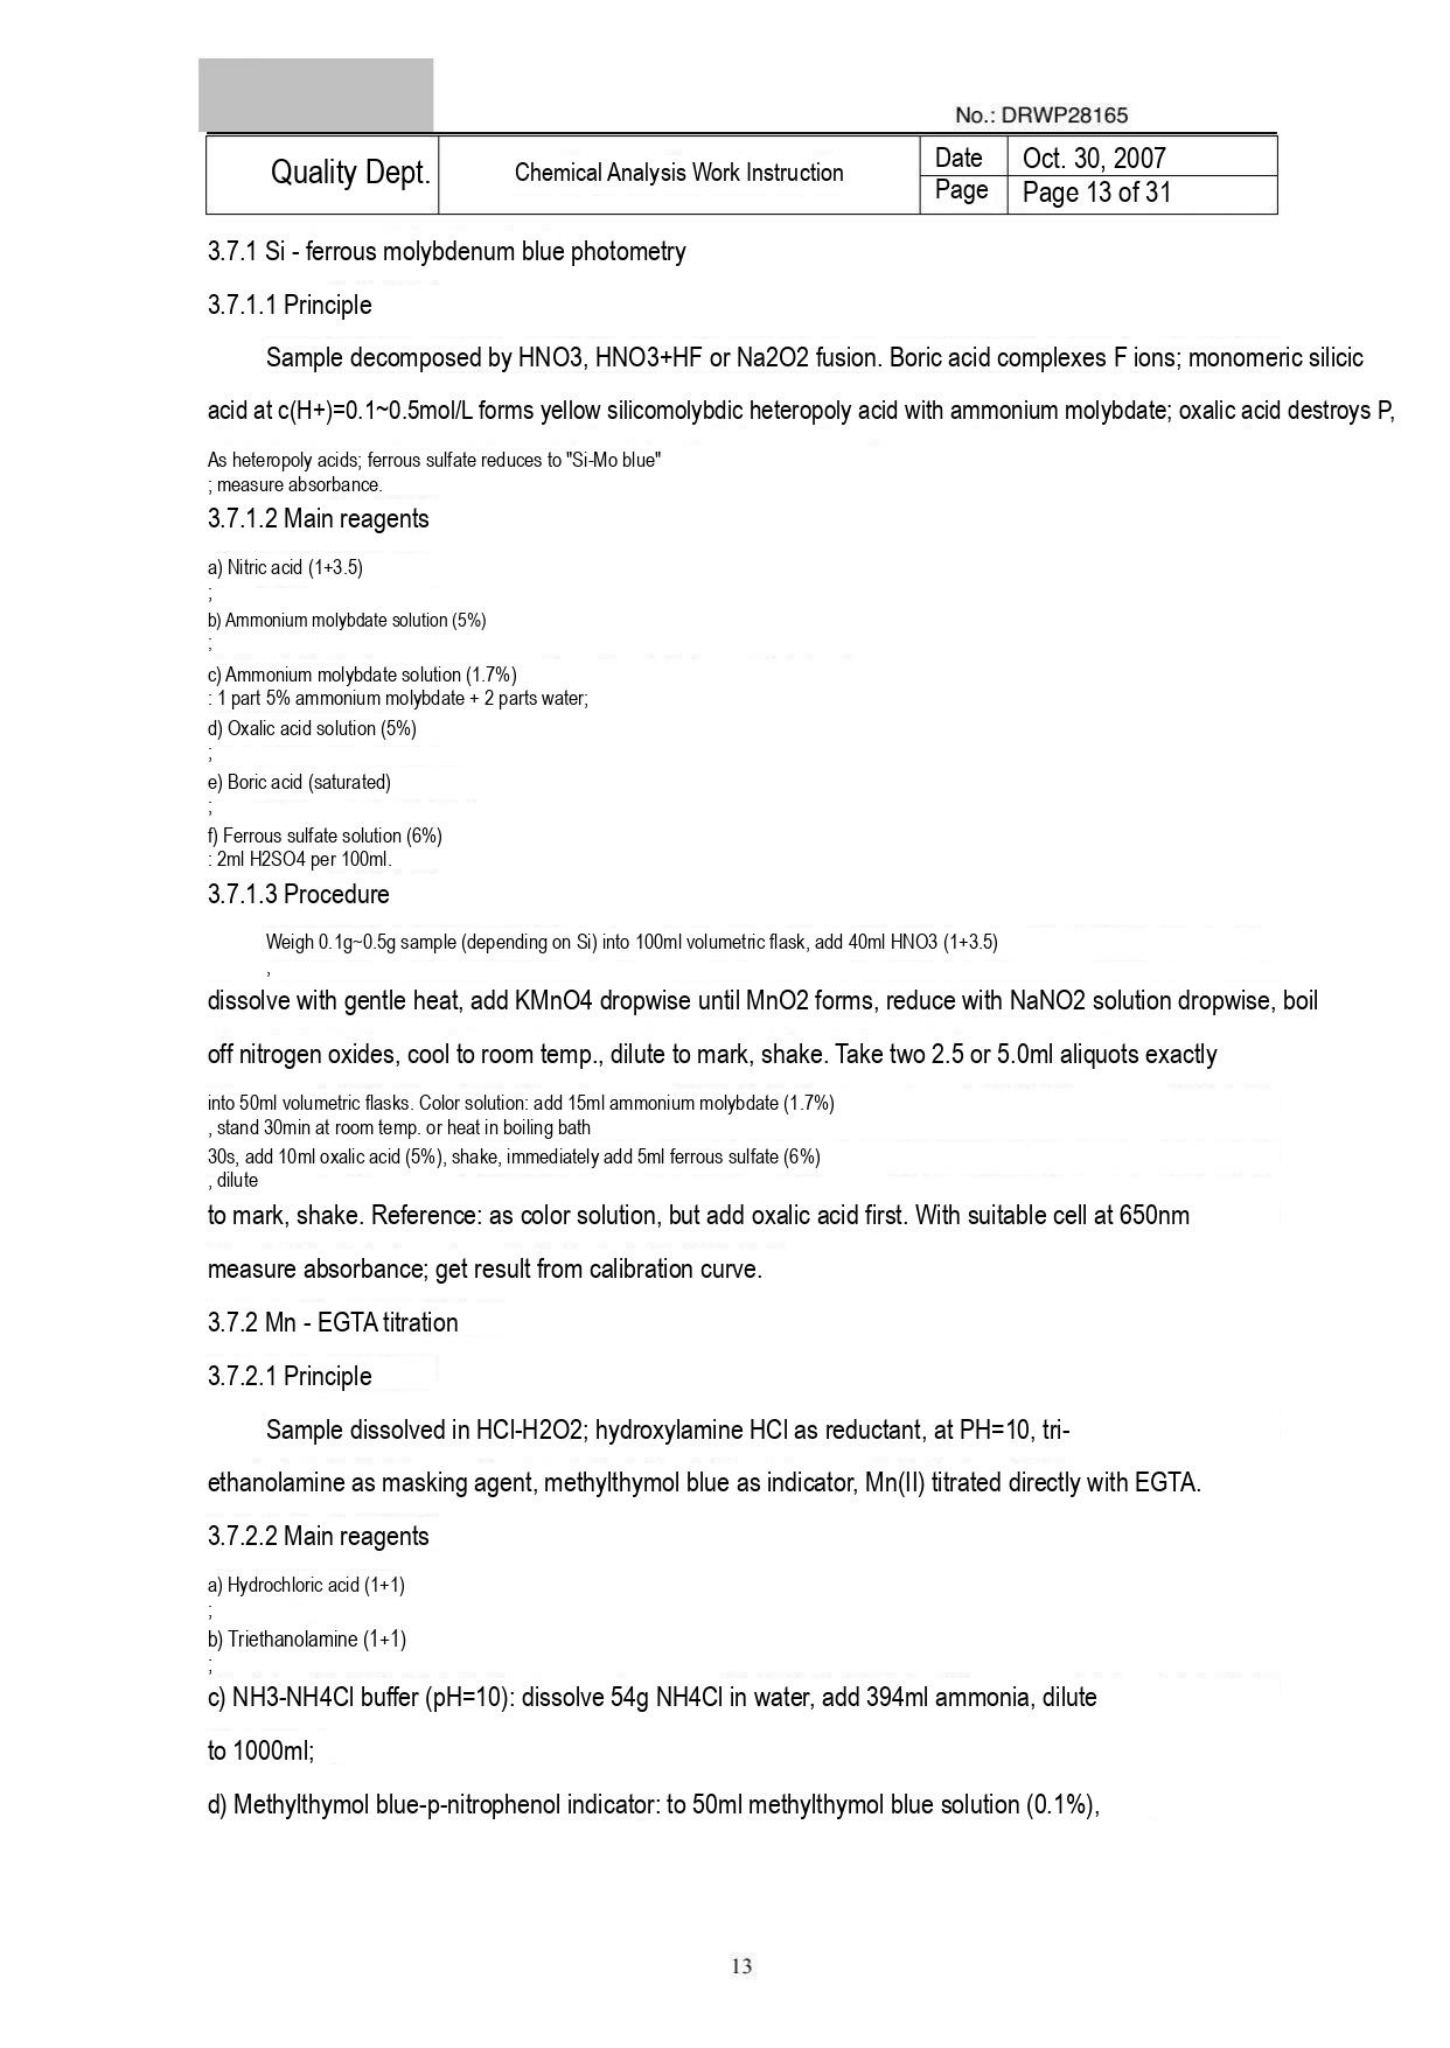No.: DRWP28165

| Quality Dept. | Chemical Analysis Work Instruction | Date | Oct. 30, 2007 |
|---|---|---|---|
| | | Page | Page 13 of 31 |

3.7.1 Si - ferrous molybdenum blue photometry

3.7.1.1 Principle

Sample decomposed by HNO3, HNO3+HF or Na2O2 fusion. Boric acid complexes F ions; monomeric silicic acid at c(H+)=0.1~0.5mol/L forms yellow silicomolybdic heteropoly acid with ammonium molybdate; oxalic acid destroys P, As heteropoly acids; ferrous sulfate reduces to "Si-Mo blue"
; measure absorbance.

3.7.1.2 Main reagents

a) Nitric acid (1+3.5)
;
b) Ammonium molybdate solution (5%)
;
c) Ammonium molybdate solution (1.7%)
: 1 part 5% ammonium molybdate + 2 parts water;
d) Oxalic acid solution (5%)
;
e) Boric acid (saturated)
;
f) Ferrous sulfate solution (6%)
: 2ml H2SO4 per 100ml.

3.7.1.3 Procedure

Weigh 0.1g~0.5g sample (depending on Si) into 100ml volumetric flask, add 40ml HNO3 (1+3.5)
,
dissolve with gentle heat, add KMnO4 dropwise until MnO2 forms, reduce with NaNO2 solution dropwise, boil off nitrogen oxides, cool to room temp., dilute to mark, shake. Take two 2.5 or 5.0ml aliquots exactly into 50ml volumetric flasks. Color solution: add 15ml ammonium molybdate (1.7%)
, stand 30min at room temp. or heat in boiling bath
30s, add 10ml oxalic acid (5%), shake, immediately add 5ml ferrous sulfate (6%)
, dilute
to mark, shake. Reference: as color solution, but add oxalic acid first. With suitable cell at 650nm measure absorbance; get result from calibration curve.

3.7.2 Mn - EGTA titration

3.7.2.1 Principle

Sample dissolved in HCl-H2O2; hydroxylamine HCl as reductant, at PH=10, tri-ethanolamine as masking agent, methylthymol blue as indicator, Mn(II) titrated directly with EGTA.

3.7.2.2 Main reagents

a) Hydrochloric acid (1+1)
;
b) Triethanolamine (1+1)
;
c) NH3-NH4Cl buffer (pH=10): dissolve 54g NH4Cl in water, add 394ml ammonia, dilute to 1000ml;

d) Methylthymol blue-p-nitrophenol indicator: to 50ml methylthymol blue solution (0.1%),

13
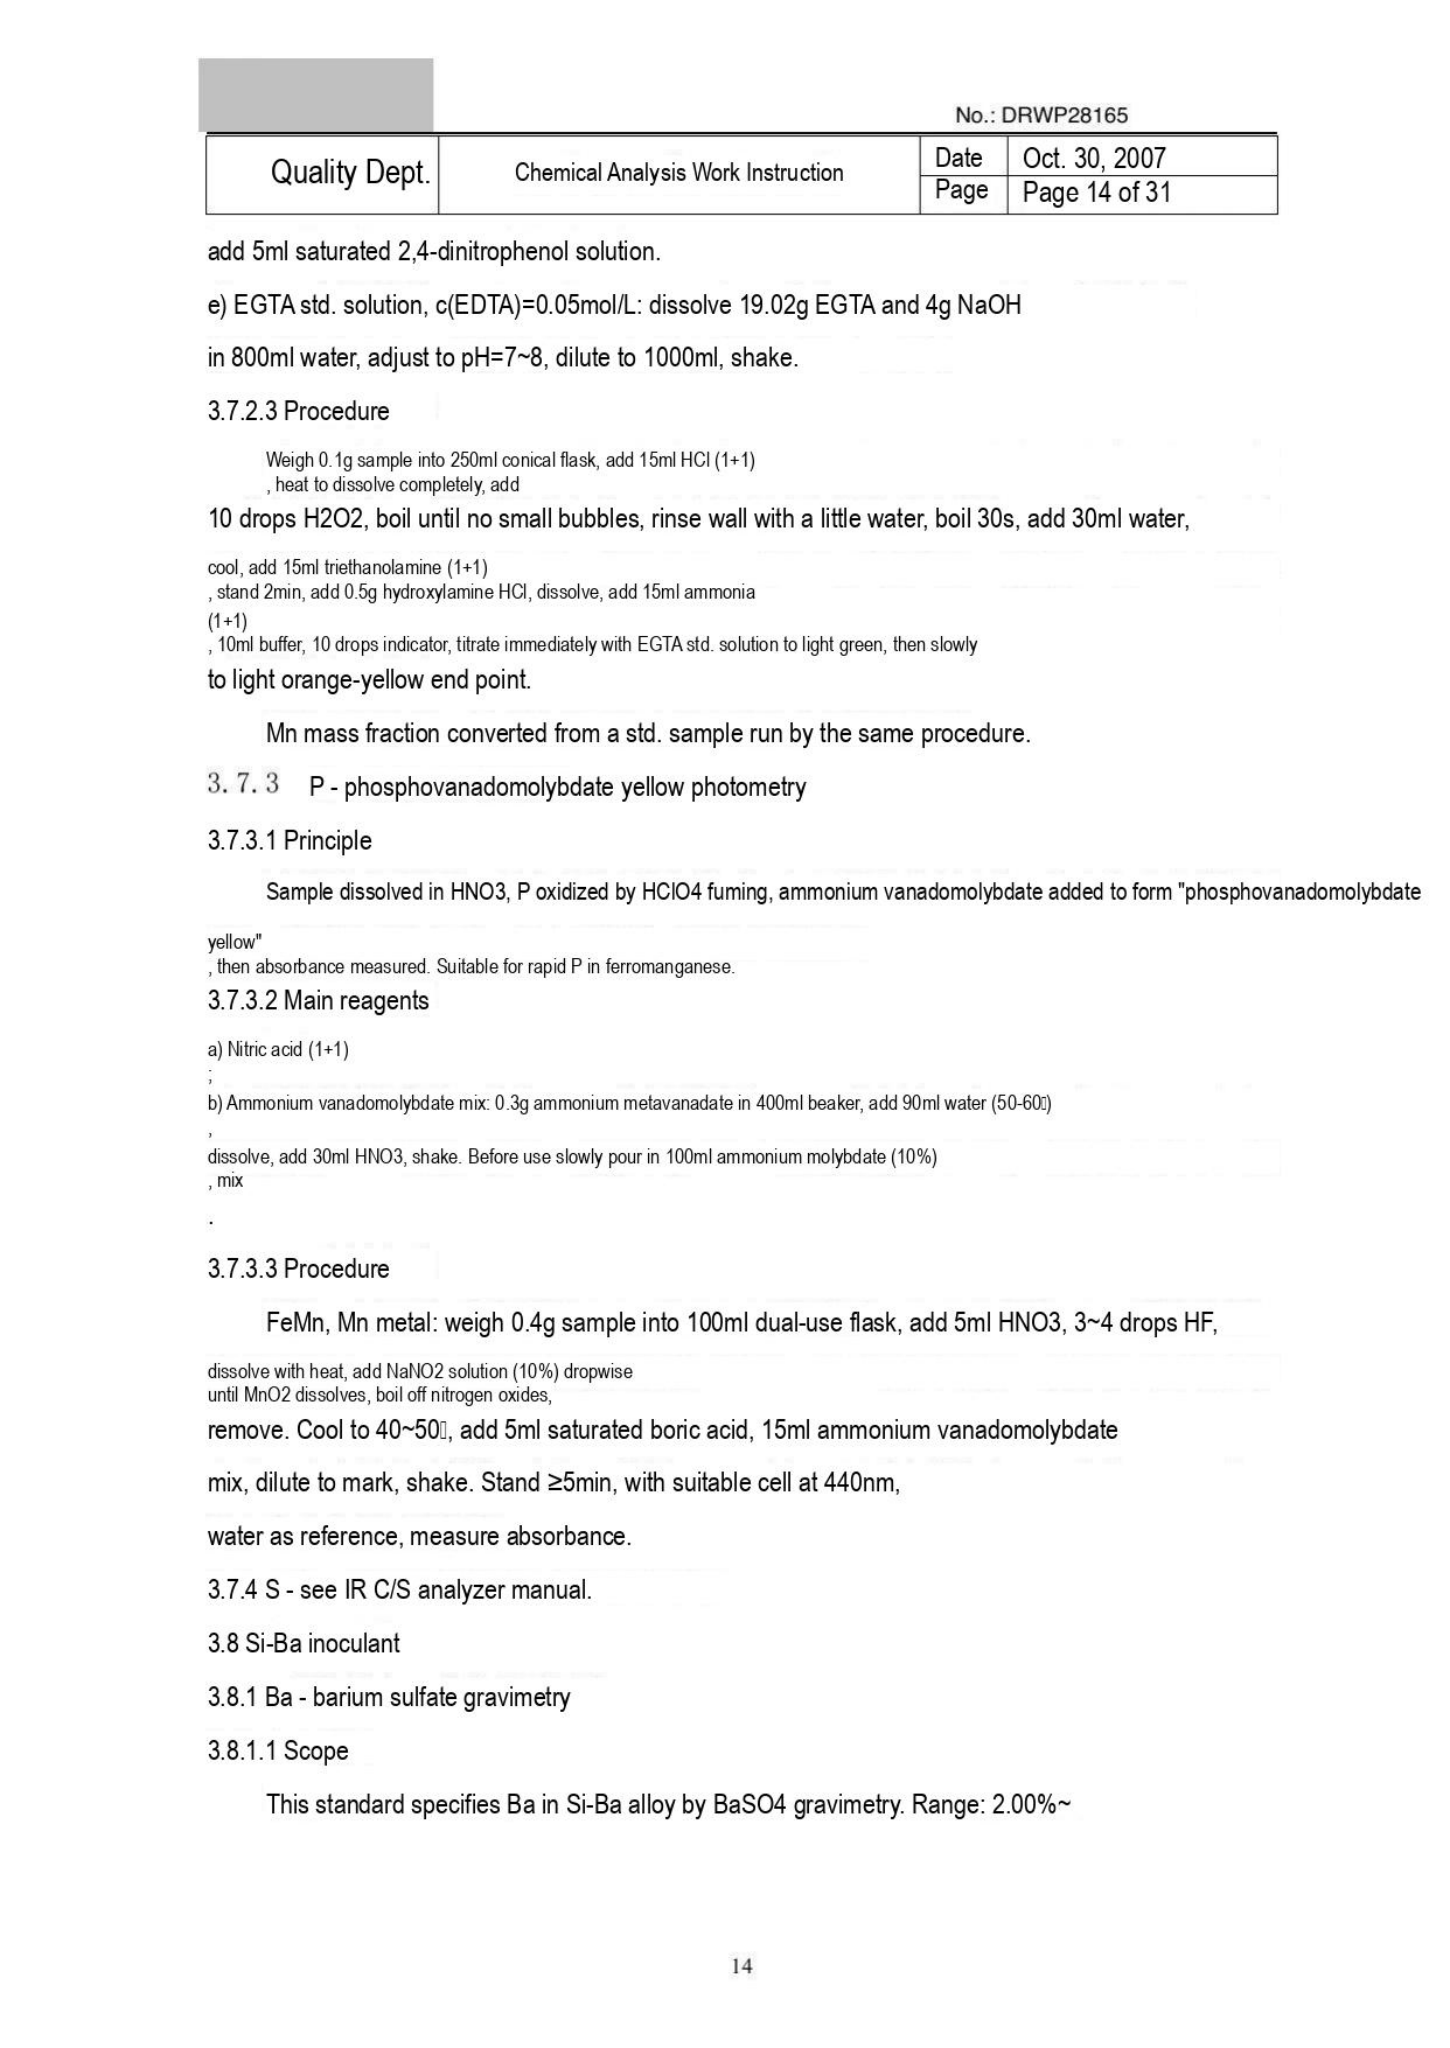No.: DRWP28165

| Quality Dept. | Chemical Analysis Work Instruction | Date | Oct. 30, 2007 |
|---|---|---|---|
| | | Page | Page 14 of 31 |

add 5ml saturated 2,4-dinitrophenol solution.

e) EGTA std. solution, c(EDTA)=0.05mol/L: dissolve 19.02g EGTA and 4g NaOH

in 800ml water, adjust to pH=7~8, dilute to 1000ml, shake.

3.7.2.3 Procedure

Weigh 0.1g sample into 250ml conical flask, add 15ml HCl (1+1)
, heat to dissolve completely, add

10 drops H2O2, boil until no small bubbles, rinse wall with a little water, boil 30s, add 30ml water,

cool, add 15ml triethanolamine (1+1)
, stand 2min, add 0.5g hydroxylamine HCl, dissolve, add 15ml ammonia
(1+1)
, 10ml buffer, 10 drops indicator, titrate immediately with EGTA std. solution to light green, then slowly

to light orange-yellow end point.

Mn mass fraction converted from a std. sample run by the same procedure.

3. 7. 3 P - phosphovanadomolybdate yellow photometry

3.7.3.1 Principle

Sample dissolved in HNO3, P oxidized by HClO4 fuming, ammonium vanadomolybdate added to form "phosphovanadomolybdate

yellow"
, then absorbance measured. Suitable for rapid P in ferromanganese.

3.7.3.2 Main reagents

a) Nitric acid (1+1)
;
b) Ammonium vanadomolybdate mix: 0.3g ammonium metavanadate in 400ml beaker, add 90ml water (50-60)
,
dissolve, add 30ml HNO3, shake. Before use slowly pour in 100ml ammonium molybdate (10%)
, mix
.

3.7.3.3 Procedure

FeMn, Mn metal: weigh 0.4g sample into 100ml dual-use flask, add 5ml HNO3, 3~4 drops HF,

dissolve with heat, add NaNO2 solution (10%) dropwise
until MnO2 dissolves, boil off nitrogen oxides,

remove. Cool to 40~50, add 5ml saturated boric acid, 15ml ammonium vanadomolybdate

mix, dilute to mark, shake. Stand ≥5min, with suitable cell at 440nm,

water as reference, measure absorbance.

3.7.4 S - see IR C/S analyzer manual.

3.8 Si-Ba inoculant

3.8.1 Ba - barium sulfate gravimetry

3.8.1.1 Scope

This standard specifies Ba in Si-Ba alloy by BaSO4 gravimetry. Range: 2.00%~

14
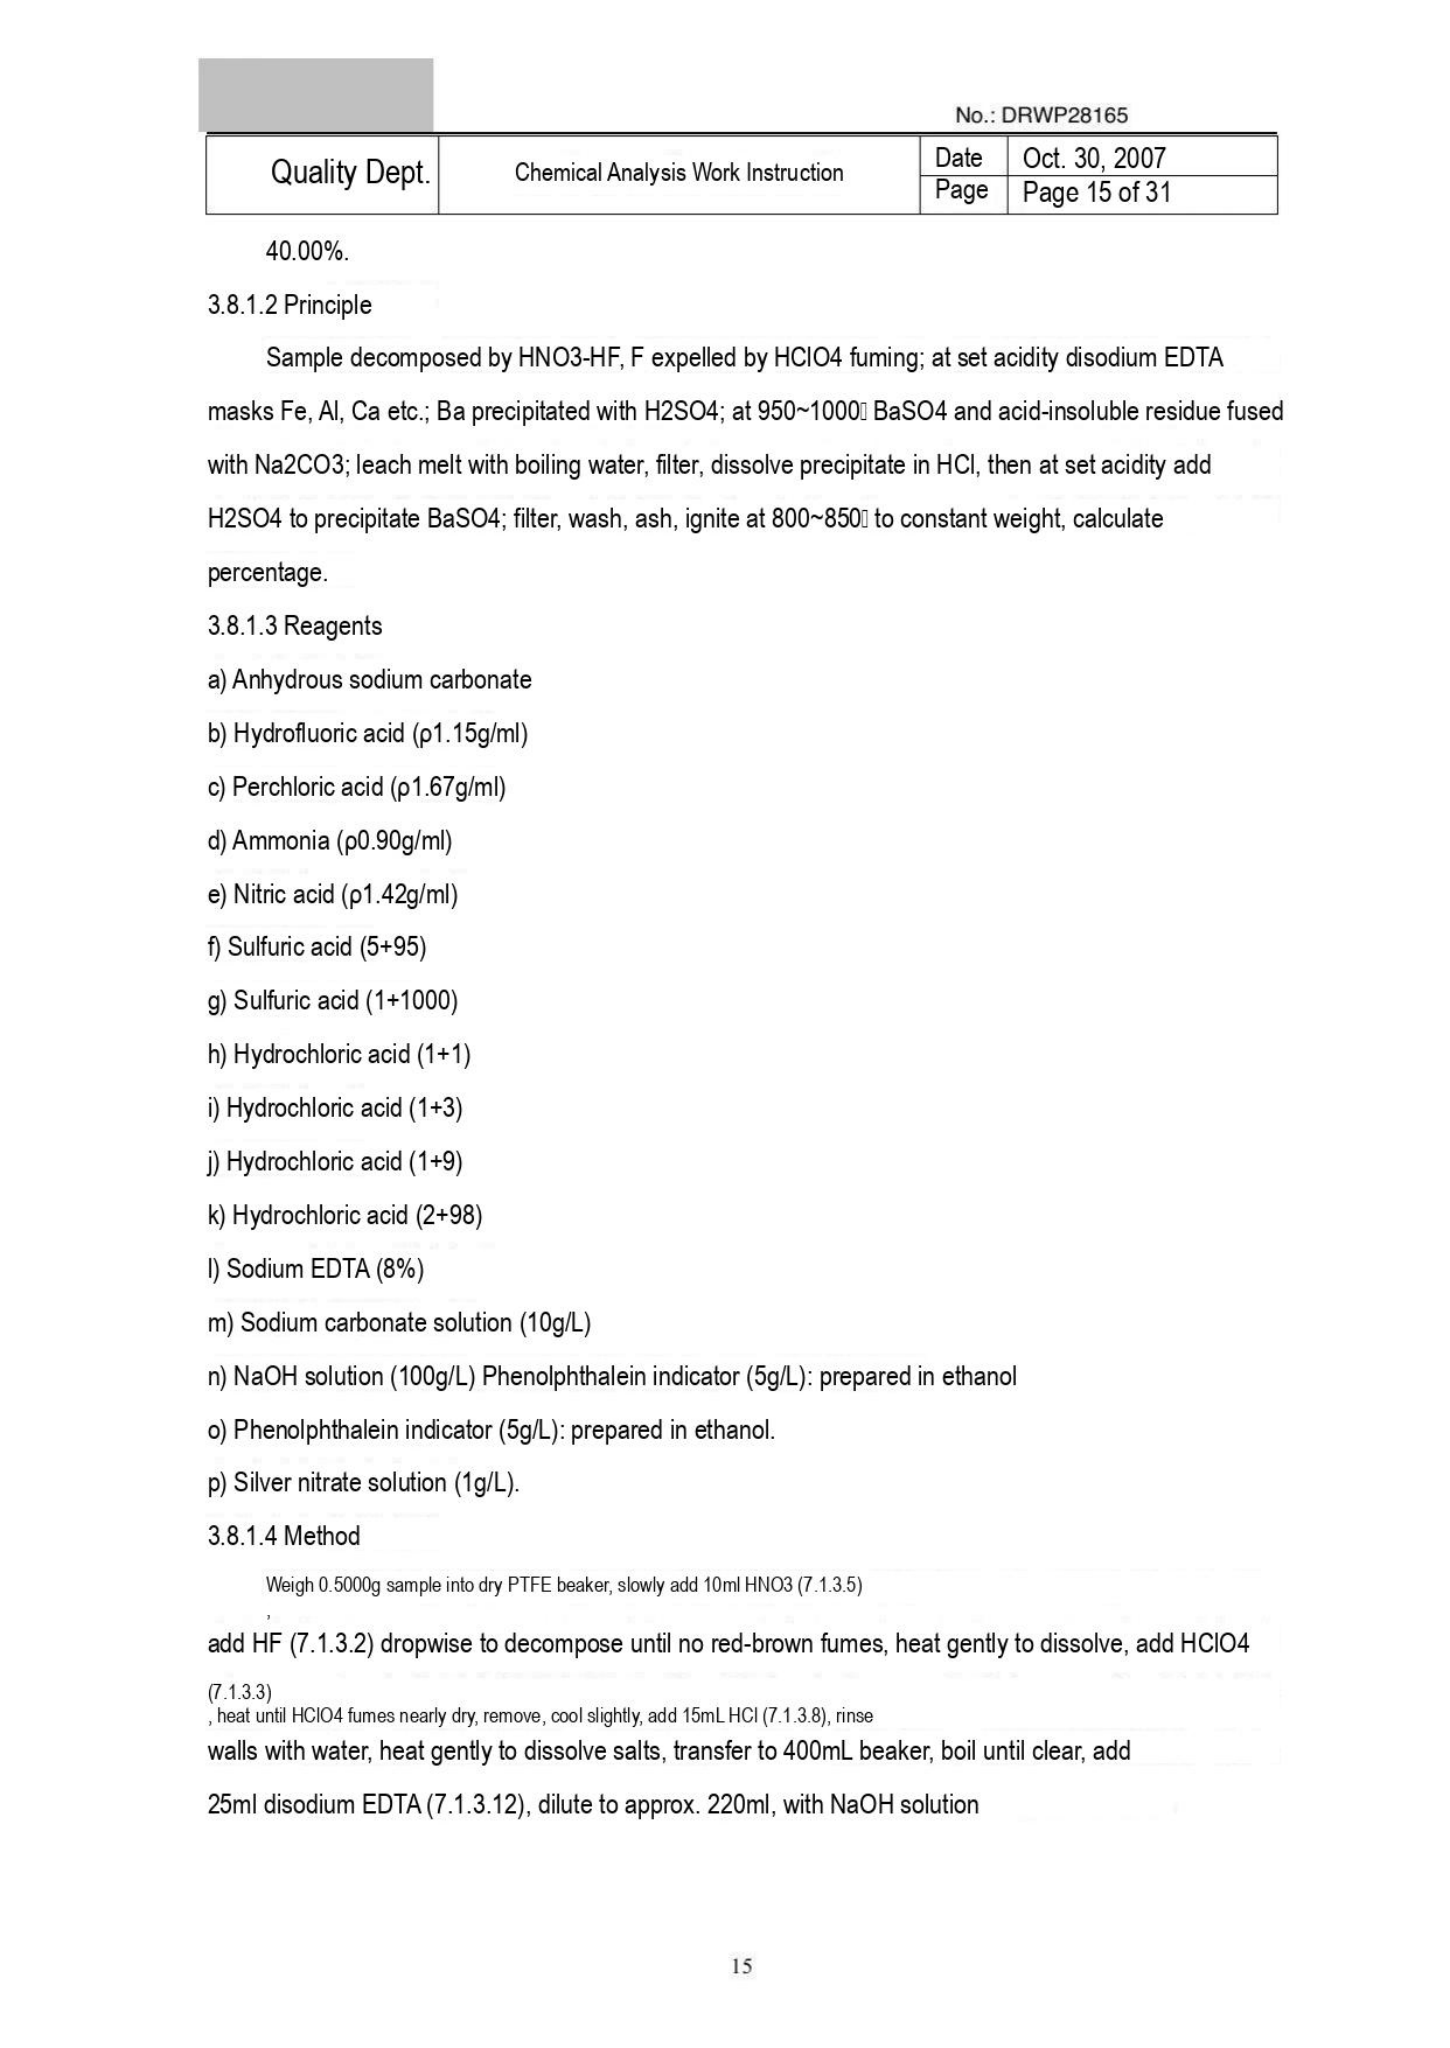No.: DRWP28165

| Quality Dept. | Chemical Analysis Work Instruction | Date | Oct. 30, 2007 |
|---|---|---|---|
| | | Page | Page 15 of 31 |

40.00%.

3.8.1.2 Principle

Sample decomposed by HNO3-HF, F expelled by HClO4 fuming; at set acidity disodium EDTA masks Fe, Al, Ca etc.; Ba precipitated with H2SO4; at 950~1000 BaSO4 and acid-insoluble residue fused with Na2CO3; leach melt with boiling water, filter, dissolve precipitate in HCl, then at set acidity add H2SO4 to precipitate BaSO4; filter, wash, ash, ignite at 800~850 to constant weight, calculate percentage.

3.8.1.3 Reagents

a) Anhydrous sodium carbonate

b) Hydrofluoric acid (ρ1.15g/ml)

c) Perchloric acid (ρ1.67g/ml)

d) Ammonia (ρ0.90g/ml)

e) Nitric acid (ρ1.42g/ml)

f) Sulfuric acid (5+95)

g) Sulfuric acid (1+1000)

h) Hydrochloric acid (1+1)

i) Hydrochloric acid (1+3)

j) Hydrochloric acid (1+9)

k) Hydrochloric acid (2+98)

l) Sodium EDTA (8%)

m) Sodium carbonate solution (10g/L)

n) NaOH solution (100g/L) Phenolphthalein indicator (5g/L): prepared in ethanol

o) Phenolphthalein indicator (5g/L): prepared in ethanol.

p) Silver nitrate solution (1g/L).

3.8.1.4 Method

Weigh 0.5000g sample into dry PTFE beaker, slowly add 10ml HNO3 (7.1.3.5)

,

add HF (7.1.3.2) dropwise to decompose until no red-brown fumes, heat gently to dissolve, add HClO4

(7.1.3.3)

, heat until HClO4 fumes nearly dry, remove, cool slightly, add 15mL HCl (7.1.3.8), rinse

walls with water, heat gently to dissolve salts, transfer to 400mL beaker, boil until clear, add

25ml disodium EDTA (7.1.3.12), dilute to approx. 220ml, with NaOH solution

15
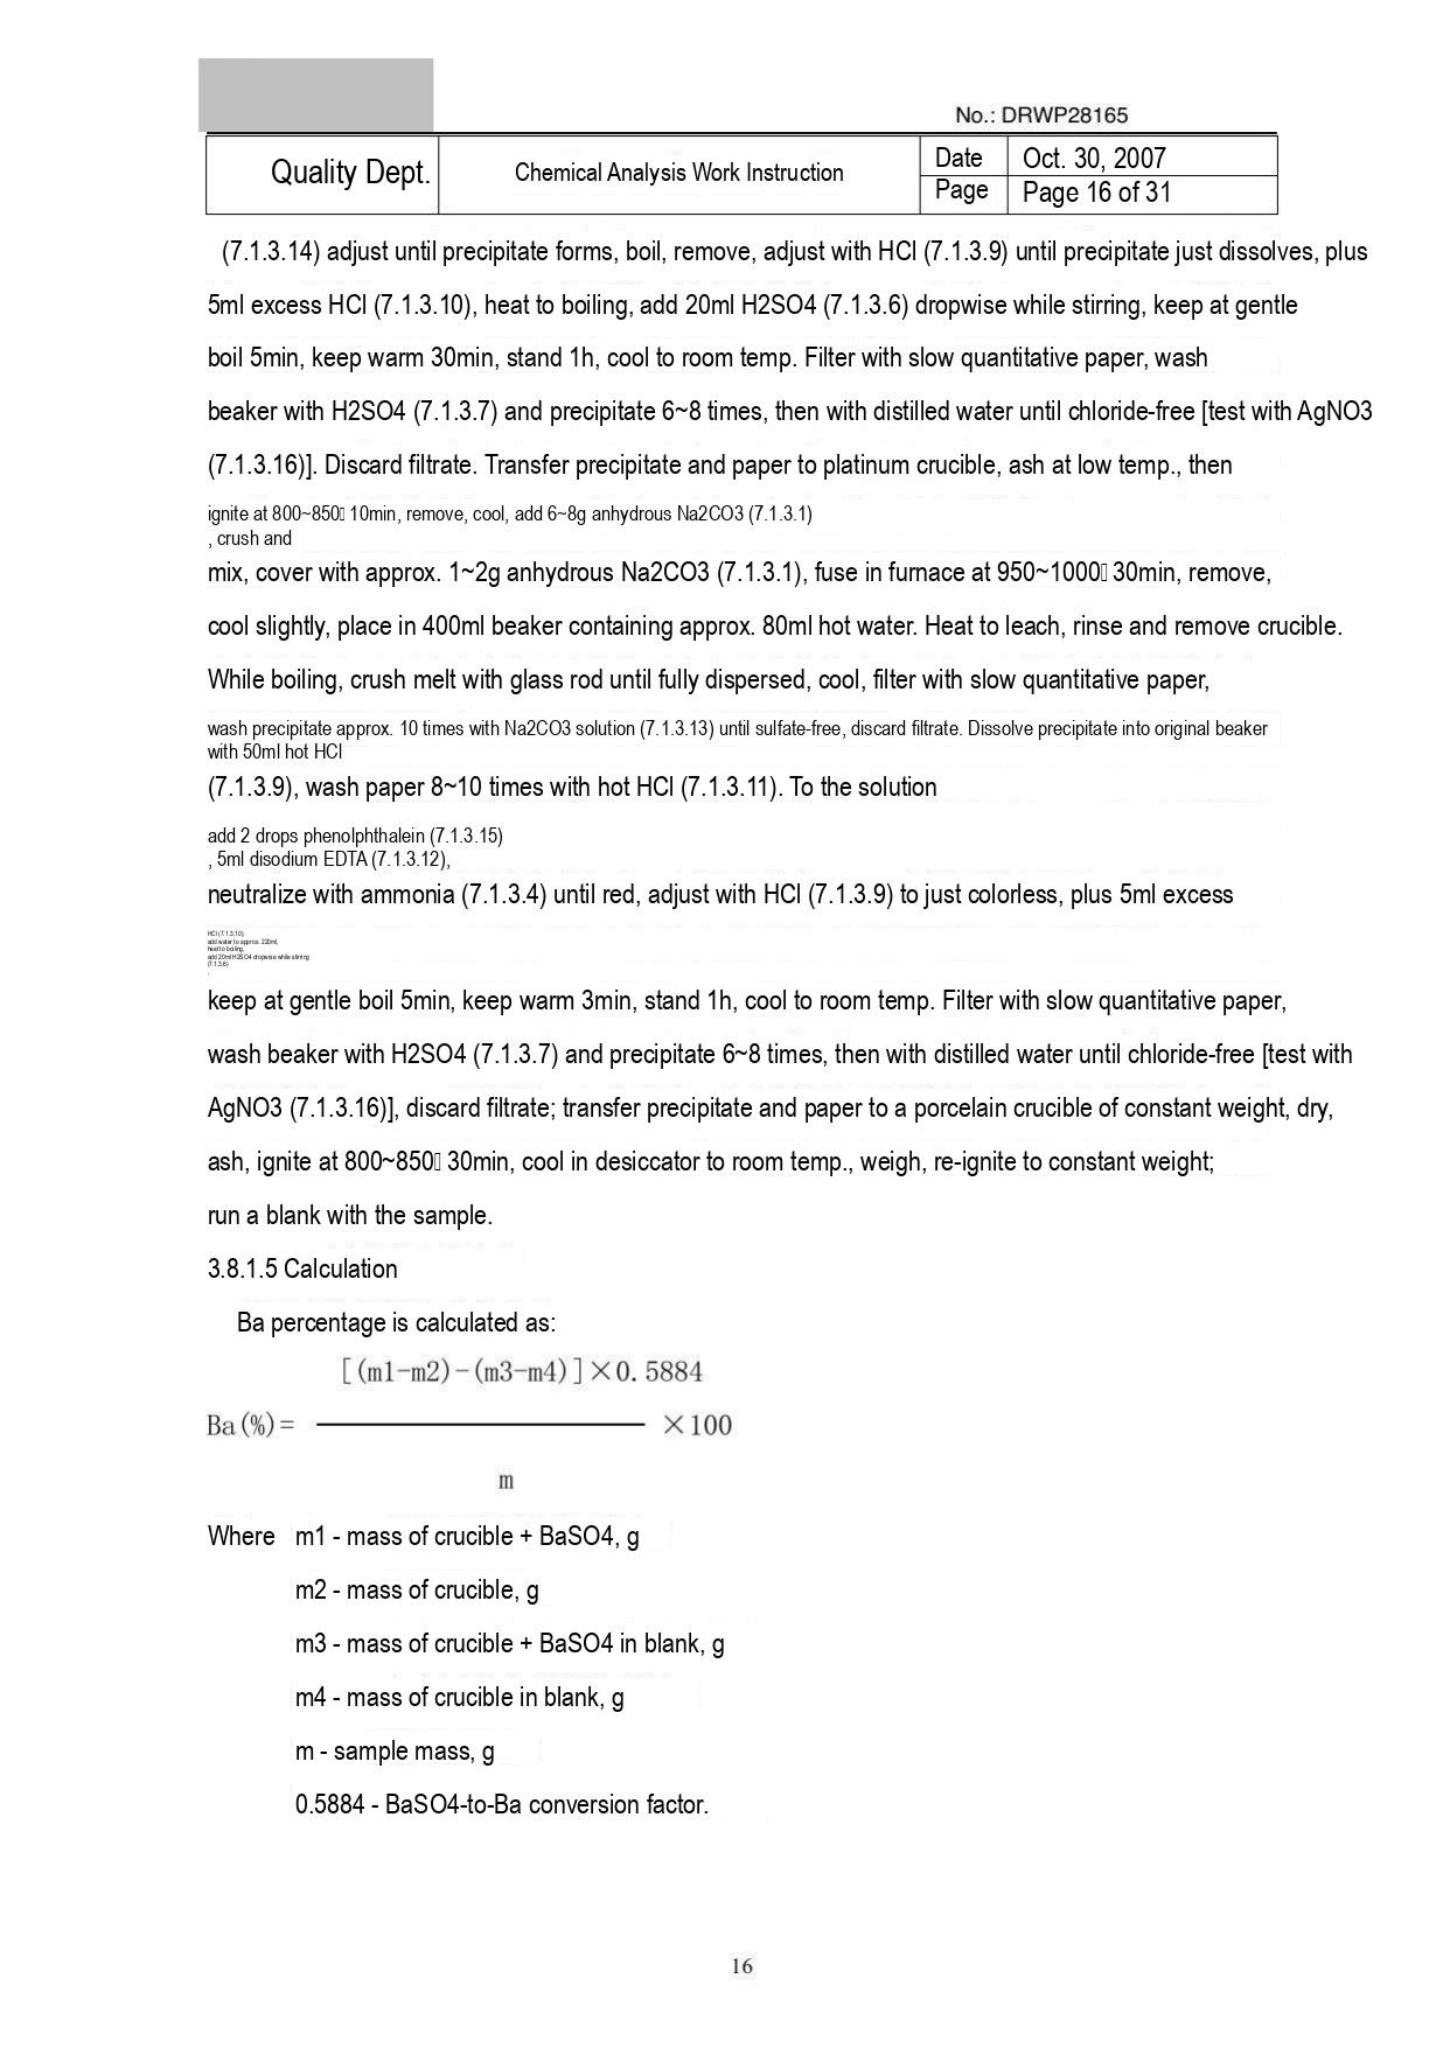No.: DRWP28165

| Quality Dept. | Chemical Analysis Work Instruction | Date | Oct. 30, 2007 |
|---|---|---|---|
| | | Page | Page 16 of 31 |

(7.1.3.14) adjust until precipitate forms, boil, remove, adjust with HCl (7.1.3.9) until precipitate just dissolves, plus 5ml excess HCl (7.1.3.10), heat to boiling, add 20ml H2SO4 (7.1.3.6) dropwise while stirring, keep at gentle boil 5min, keep warm 30min, stand 1h, cool to room temp. Filter with slow quantitative paper, wash beaker with H2SO4 (7.1.3.7) and precipitate 6~8 times, then with distilled water until chloride-free [test with AgNO3 (7.1.3.16)]. Discard filtrate. Transfer precipitate and paper to platinum crucible, ash at low temp., then

ignite at 800~850 10min, remove, cool, add 6~8g anhydrous Na2CO3 (7.1.3.1)
, crush and

mix, cover with approx. 1~2g anhydrous Na2CO3 (7.1.3.1), fuse in furnace at 950~1000 30min, remove, cool slightly, place in 400ml beaker containing approx. 80ml hot water. Heat to leach, rinse and remove crucible. While boiling, crush melt with glass rod until fully dispersed, cool, filter with slow quantitative paper,

wash precipitate approx. 10 times with Na2CO3 solution (7.1.3.13) until sulfate-free, discard filtrate. Dissolve precipitate into original beaker with 50ml hot HCl

(7.1.3.9), wash paper 8~10 times with hot HCl (7.1.3.11). To the solution

add 2 drops phenolphthalein (7.1.3.15)
, 5ml disodium EDTA (7.1.3.12),

neutralize with ammonia (7.1.3.4) until red, adjust with HCl (7.1.3.9) to just colorless, plus 5ml excess

HCl (7.1.3.10)
add water to approx. 220ml,
heat to boiling,
add 20ml H2SO4 dropwise while stirring
(7.1.3.6)

keep at gentle boil 5min, keep warm 3min, stand 1h, cool to room temp. Filter with slow quantitative paper, wash beaker with H2SO4 (7.1.3.7) and precipitate 6~8 times, then with distilled water until chloride-free [test with AgNO3 (7.1.3.16)], discard filtrate; transfer precipitate and paper to a porcelain crucible of constant weight, dry, ash, ignite at 800~850 30min, cool in desiccator to room temp., weigh, re-ignite to constant weight; run a blank with the sample.

3.8.1.5 Calculation

Ba percentage is calculated as:

Ba (%) = [(m1−m2)−(m3−m4)]×0.5884 / m ×100

Where m1 - mass of crucible + BaSO4, g

m2 - mass of crucible, g

m3 - mass of crucible + BaSO4 in blank, g

m4 - mass of crucible in blank, g

m - sample mass, g

0.5884 - BaSO4-to-Ba conversion factor.

16
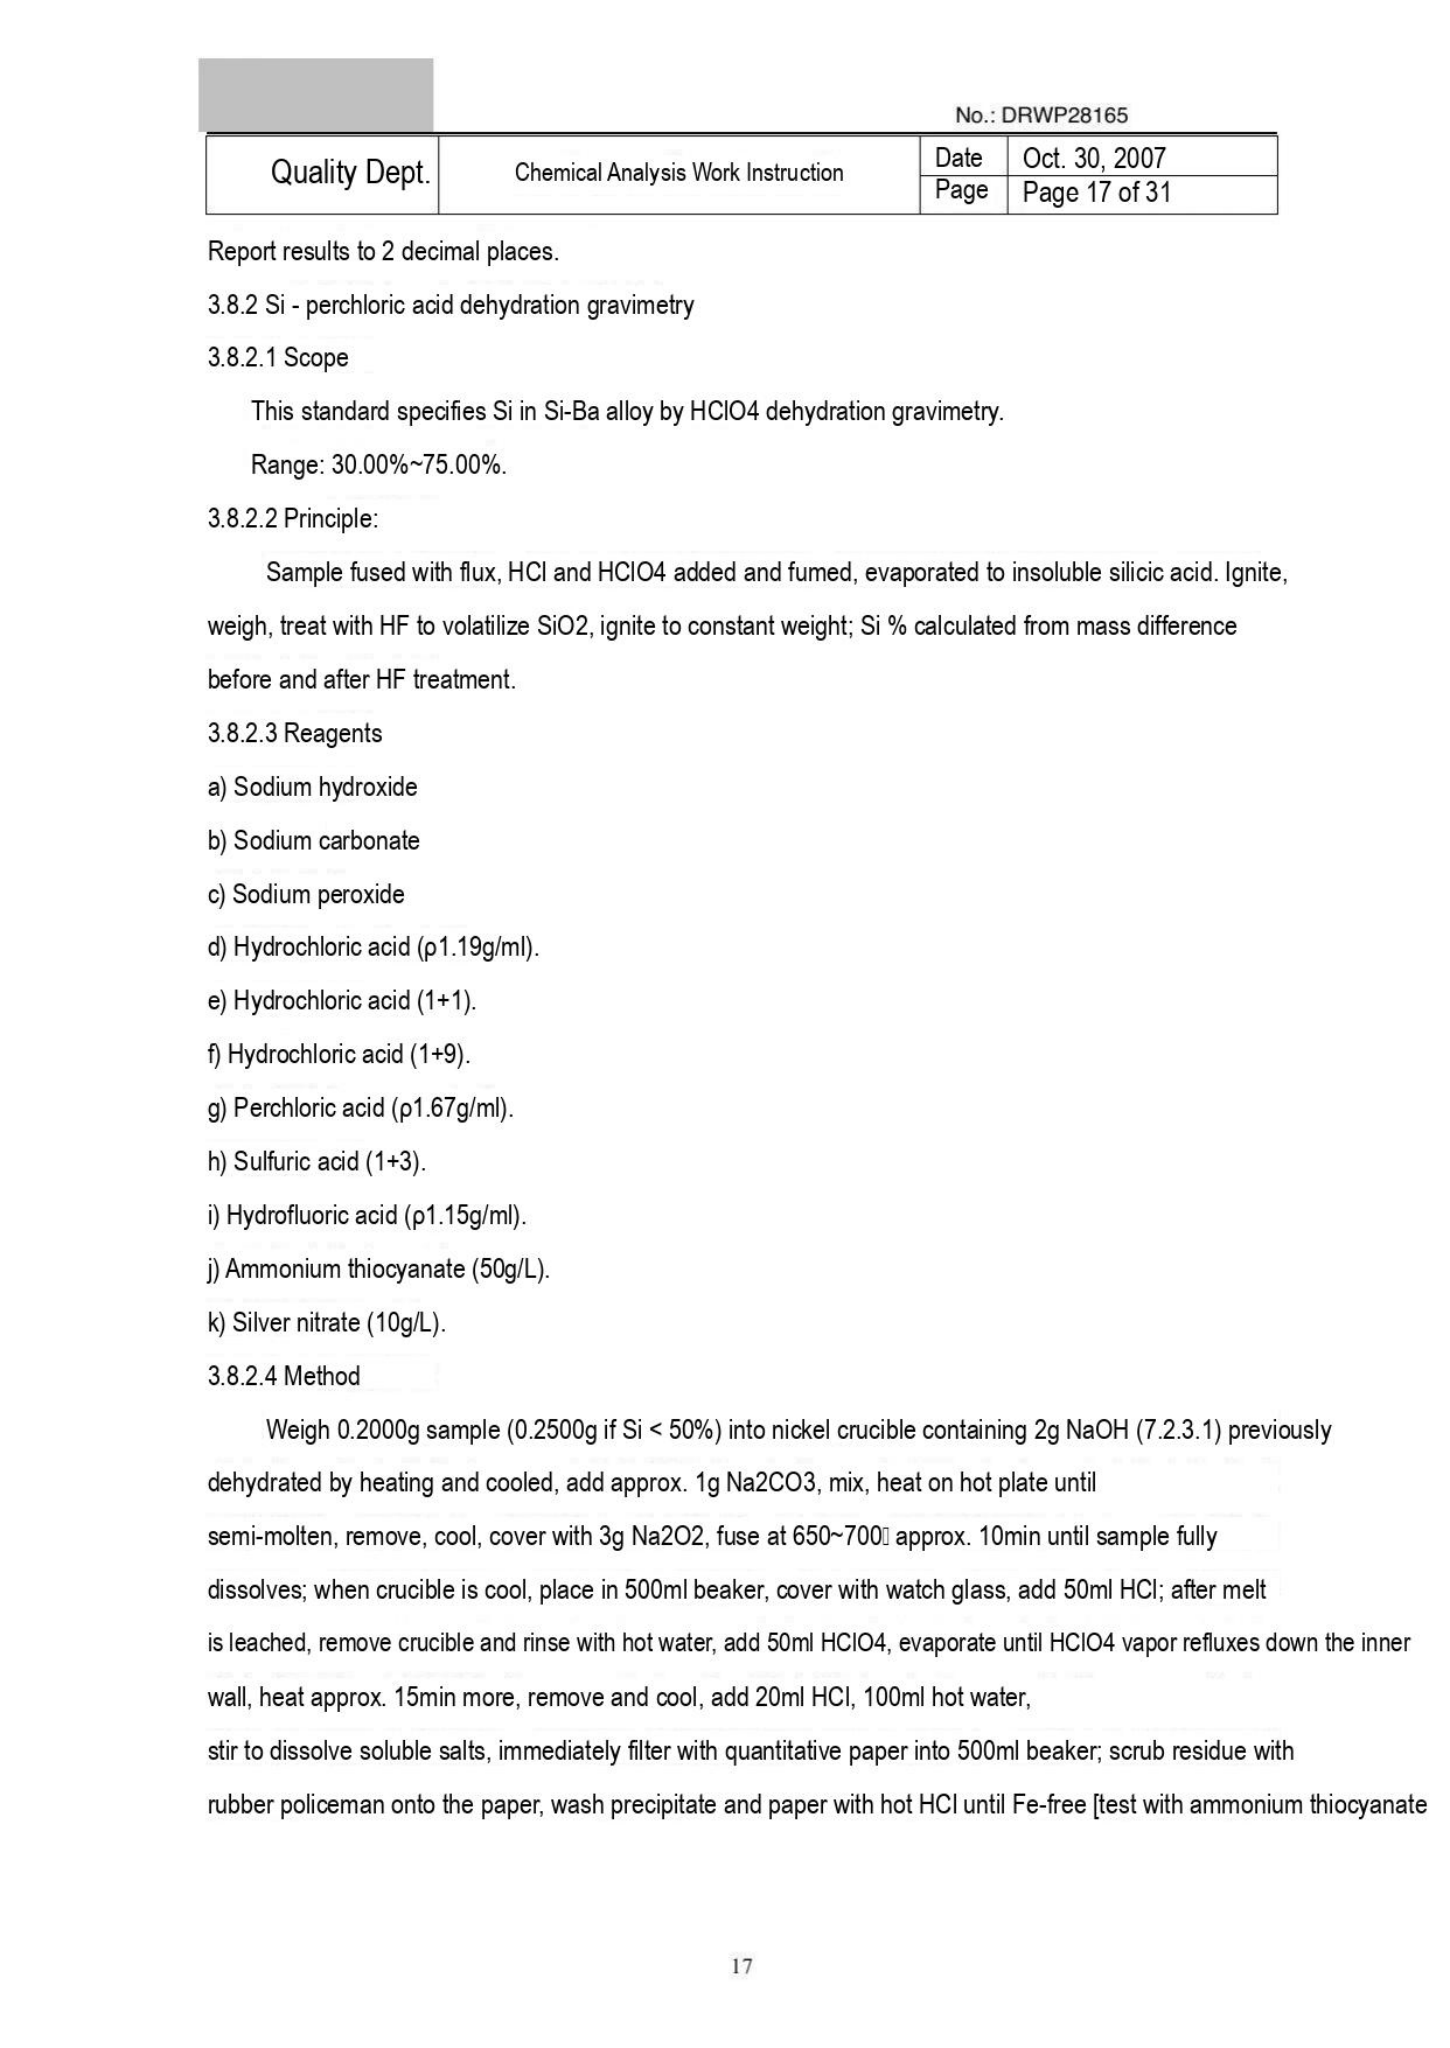No.: DRWP28165

| Quality Dept. | Chemical Analysis Work Instruction | Date | Oct. 30, 2007 |
|---|---|---|---|
| | | Page | Page 17 of 31 |

Report results to 2 decimal places.

3.8.2 Si - perchloric acid dehydration gravimetry

3.8.2.1 Scope

This standard specifies Si in Si-Ba alloy by HClO4 dehydration gravimetry.

Range: 30.00%~75.00%.

3.8.2.2 Principle:

Sample fused with flux, HCl and HClO4 added and fumed, evaporated to insoluble silicic acid. Ignite, weigh, treat with HF to volatilize SiO2, ignite to constant weight; Si % calculated from mass difference before and after HF treatment.

3.8.2.3 Reagents

a) Sodium hydroxide

b) Sodium carbonate

c) Sodium peroxide

d) Hydrochloric acid (ρ1.19g/ml).

e) Hydrochloric acid (1+1).

f) Hydrochloric acid (1+9).

g) Perchloric acid (ρ1.67g/ml).

h) Sulfuric acid (1+3).

i) Hydrofluoric acid (ρ1.15g/ml).

j) Ammonium thiocyanate (50g/L).

k) Silver nitrate (10g/L).

3.8.2.4 Method

Weigh 0.2000g sample (0.2500g if Si < 50%) into nickel crucible containing 2g NaOH (7.2.3.1) previously dehydrated by heating and cooled, add approx. 1g Na2CO3, mix, heat on hot plate until semi-molten, remove, cool, cover with 3g Na2O2, fuse at 650~700 approx. 10min until sample fully dissolves; when crucible is cool, place in 500ml beaker, cover with watch glass, add 50ml HCl; after melt is leached, remove crucible and rinse with hot water, add 50ml HClO4, evaporate until HClO4 vapor refluxes down the inner wall, heat approx. 15min more, remove and cool, add 20ml HCl, 100ml hot water, stir to dissolve soluble salts, immediately filter with quantitative paper into 500ml beaker; scrub residue with rubber policeman onto the paper, wash precipitate and paper with hot HCl until Fe-free [test with ammonium thiocyanate

17
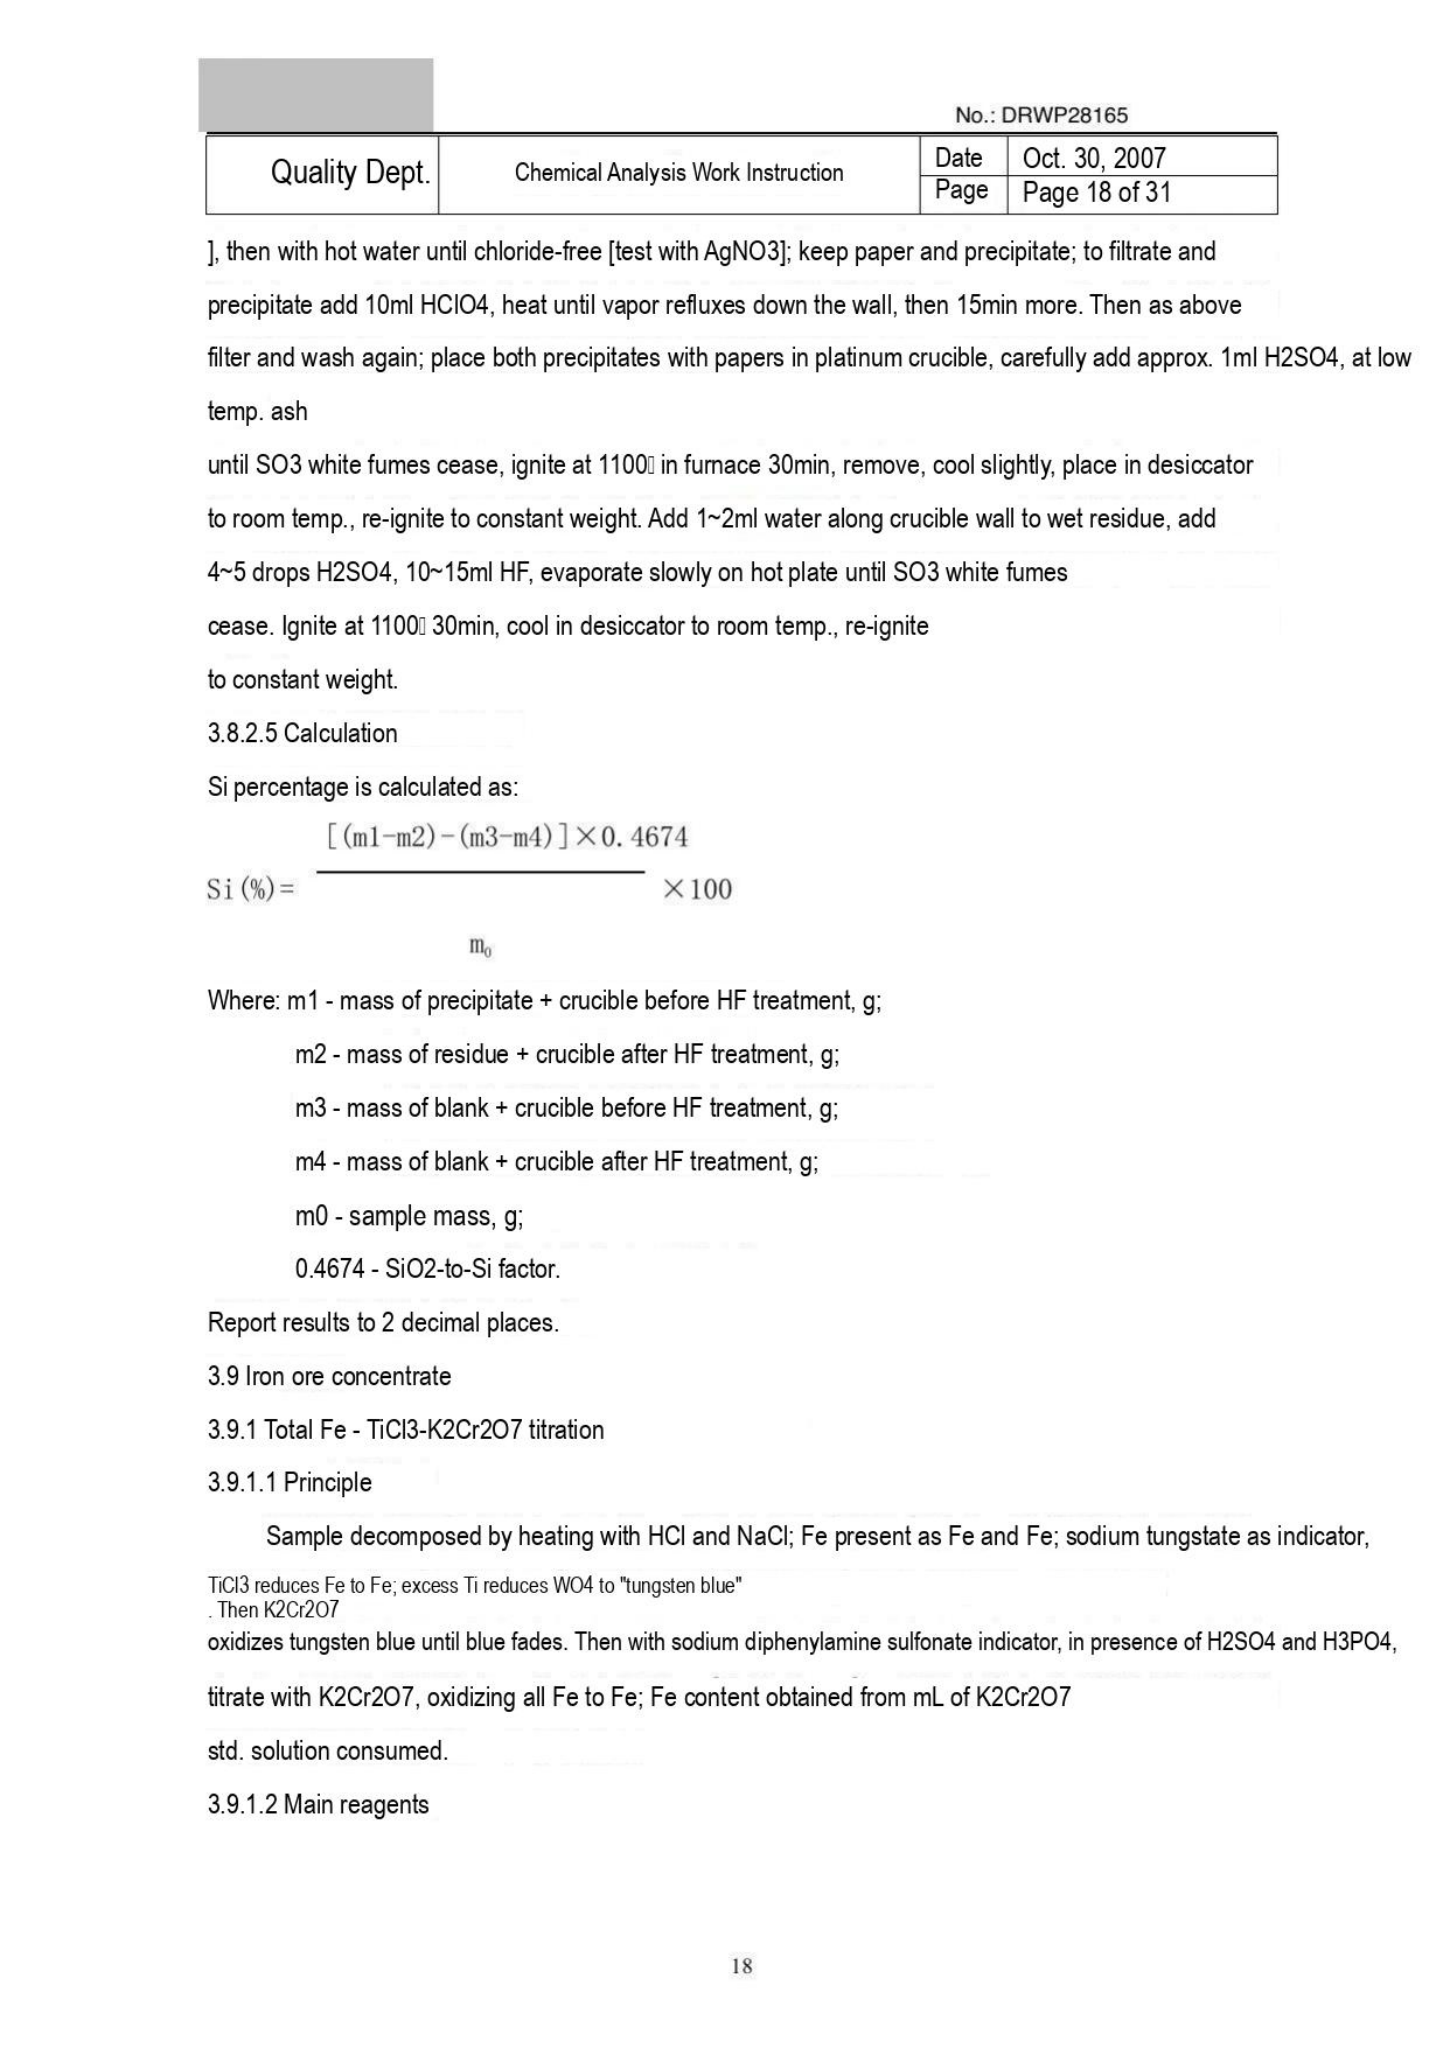No.: DRWP28165

| Quality Dept. | Chemical Analysis Work Instruction | Date | Oct. 30, 2007 |
|---|---|---|---|
| | | Page | Page 18 of 31 |

], then with hot water until chloride-free [test with AgNO3]; keep paper and precipitate; to filtrate and precipitate add 10ml HClO4, heat until vapor refluxes down the wall, then 15min more. Then as above filter and wash again; place both precipitates with papers in platinum crucible, carefully add approx. 1ml H2SO4, at low temp. ash

until SO3 white fumes cease, ignite at 1100 in furnace 30min, remove, cool slightly, place in desiccator to room temp., re-ignite to constant weight. Add 1~2ml water along crucible wall to wet residue, add 4~5 drops H2SO4, 10~15ml HF, evaporate slowly on hot plate until SO3 white fumes cease. Ignite at 1100 30min, cool in desiccator to room temp., re-ignite to constant weight.

3.8.2.5 Calculation

Si percentage is calculated as:

Si (%) = [(m1-m2)-(m3-m4)]×0.4674 / m₀ ×100

Where: m1 - mass of precipitate + crucible before HF treatment, g;

m2 - mass of residue + crucible after HF treatment, g;

m3 - mass of blank + crucible before HF treatment, g;

m4 - mass of blank + crucible after HF treatment, g;

m0 - sample mass, g;

0.4674 - SiO2-to-Si factor.

Report results to 2 decimal places.

3.9 Iron ore concentrate

3.9.1 Total Fe - TiCl3-K2Cr2O7 titration

3.9.1.1 Principle

Sample decomposed by heating with HCl and NaCl; Fe present as Fe and Fe; sodium tungstate as indicator,

TiCl3 reduces Fe to Fe; excess Ti reduces WO4 to "tungsten blue"
. Then K2Cr2O7
oxidizes tungsten blue until blue fades. Then with sodium diphenylamine sulfonate indicator, in presence of H2SO4 and H3PO4, titrate with K2Cr2O7, oxidizing all Fe to Fe; Fe content obtained from mL of K2Cr2O7 std. solution consumed.

3.9.1.2 Main reagents

18